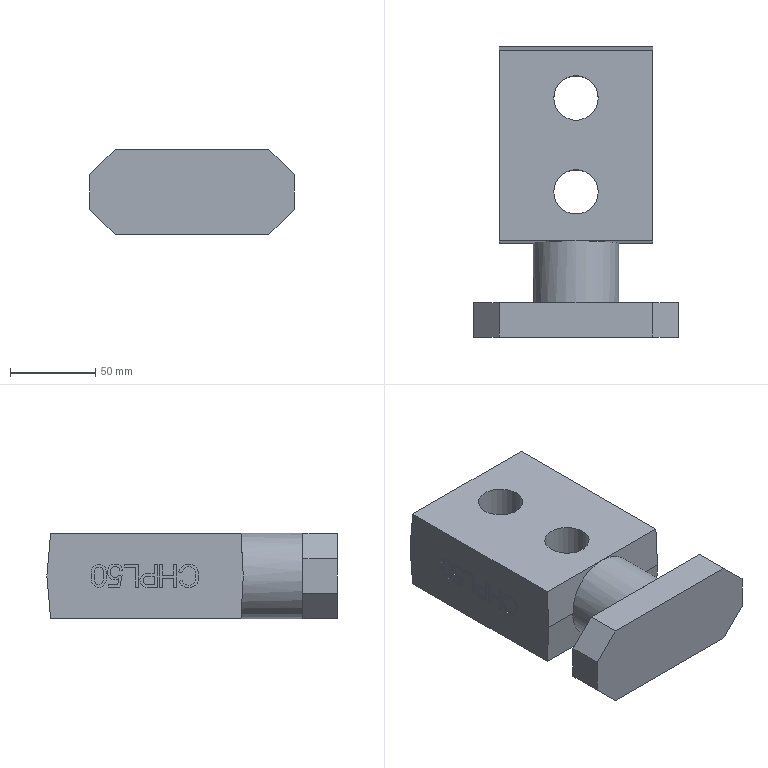Part | NX | features MI_CHPL_0745 2 | 1 solid | 99 faces | box 120 x 170 x 50 mm | volume 637321 mm3 | plane 77 | cylinder 22 | commonest cylinder face diameters 26 x2 4.776 x1 5.395 x1 5.672 x1 5.699 x1 6.768 x1